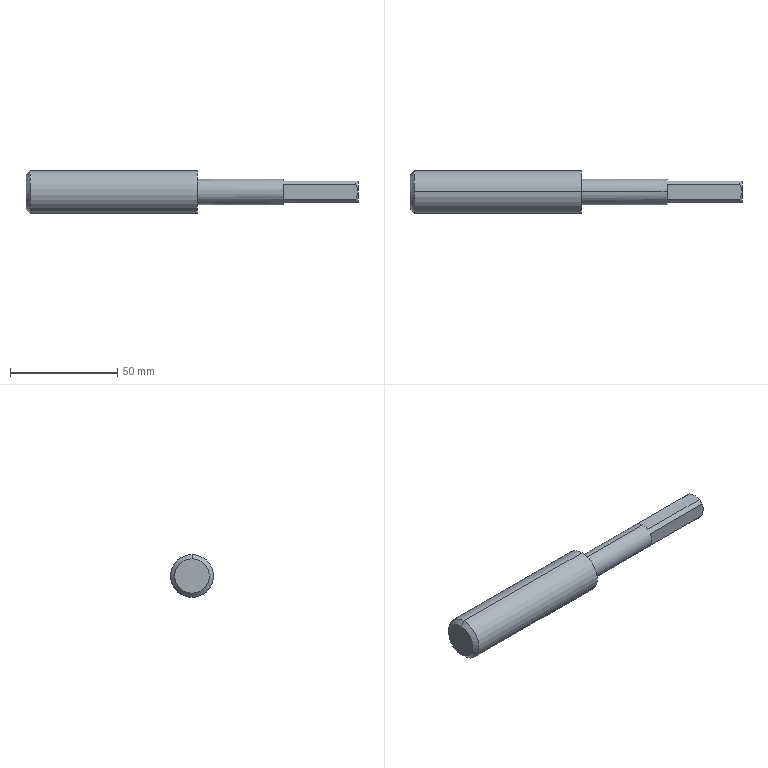Part | SolidWorks | features Chamfer 2, ICE 1, Revolution 1 | 1 solid | 21 faces | box 155 x 20 x 20 mm | volume 32861 mm3 | plane 11 | cone 6 | cylinder 4 | commonest cylinder face diameters 12 x2 20 x2
STEP:
#1=CARTESIAN_POINT('',(0.,0.,8.));
#2=VERTEX_POINT('',#1);
#3=CARTESIAN_POINT('',(0.,0.,-8.));
#4=VERTEX_POINT('',#3);
#5=CARTESIAN_POINT('',(0.,0.,0.));
#6=DIRECTION('',(-1.,0.,0.));
#7=DIRECTION('',(0.,0.,-1.));
#8=AXIS2_PLACEMENT_3D('',#5,#6,#7);
#9=CIRCLE('',#8,8.);
#10=EDGE_CURVE('',#2,#4,#9,.T.);
#11=ORIENTED_EDGE('',*,*,#10,.F.);
#12=CARTESIAN_POINT('',(2.,0.,10.));
#13=VERTEX_POINT('',#12);
#14=CARTESIAN_POINT('',(0.,0.,8.));
#15=DIRECTION('',(0.7071,0.,0.7071));
#16=VECTOR('',#15,1000.);
#17=LINE('',#14,#16);
#18=EDGE_CURVE('',#2,#13,#17,.T.);
#19=ORIENTED_EDGE('',*,*,#18,.T.);
#20=CARTESIAN_POINT('',(2.,0.,-10.));
#21=VERTEX_POINT('',#20);
#22=CARTESIAN_POINT('',(2.,0.,0.));
#23=DIRECTION('',(1.,0.,0.));
#24=DIRECTION('',(0.,0.,-1.));
#25=AXIS2_PLACEMENT_3D('',#22,#23,#24);
#26=CIRCLE('',#25,10.);
#27=EDGE_CURVE('',#21,#13,#26,.T.);
#28=ORIENTED_EDGE('',*,*,#27,.F.);
#29=CARTESIAN_POINT('',(0.,0.,-8.));
#30=DIRECTION('',(0.7071,0.,-0.7071));
#31=VECTOR('',#30,1000.);
#32=LINE('',#29,#31);
#33=EDGE_CURVE('',#4,#21,#32,.T.);
#34=ORIENTED_EDGE('',*,*,#33,.F.);
#35=EDGE_LOOP('',(#11,#19,#28,#34));
#36=FACE_OUTER_BOUND('',#35,.T.);
#37=CARTESIAN_POINT('',(0.,0.,0.));
#38=DIRECTION('',(1.,0.,0.));
#39=DIRECTION('',(0.,0.,-1.));
#40=AXIS2_PLACEMENT_3D('',#37,#38,#39);
#41=CONICAL_SURFACE('',#40,8.,0.7854);
#42=ADVANCED_FACE('',(#36),#41,.T.);
#43=CARTESIAN_POINT('',(80.,0.,10.));
#44=VERTEX_POINT('',#43);
#45=CARTESIAN_POINT('',(80.,0.,-10.));
#46=VERTEX_POINT('',#45);
#47=CARTESIAN_POINT('',(80.,0.,0.));
#48=DIRECTION('',(-1.,0.,0.));
#49=DIRECTION('',(0.,0.,1.));
#50=AXIS2_PLACEMENT_3D('',#47,#48,#49);
#51=CIRCLE('',#50,10.);
#52=EDGE_CURVE('',#44,#46,#51,.T.);
#53=ORIENTED_EDGE('',*,*,#52,.T.);
#54=CARTESIAN_POINT('',(0.,0.,-10.));
#55=DIRECTION('',(-1.,0.,0.));
#56=VECTOR('',#55,1000.);
#57=LINE('',#54,#56);
#58=EDGE_CURVE('',#46,#21,#57,.T.);
#59=ORIENTED_EDGE('',*,*,#58,.T.);
#60=ORIENTED_EDGE('',*,*,#27,.T.);
#61=CARTESIAN_POINT('',(0.,0.,10.));
#62=DIRECTION('',(-1.,0.,0.));
#63=VECTOR('',#62,1000.);
#64=LINE('',#61,#63);
#65=EDGE_CURVE('',#44,#13,#64,.T.);
#66=ORIENTED_EDGE('',*,*,#65,.F.);
#67=EDGE_LOOP('',(#53,#59,#60,#66));
#68=FACE_OUTER_BOUND('',#67,.T.);
#69=CARTESIAN_POINT('',(0.,0.,0.));
#70=DIRECTION('',(-1.,0.,0.));
#71=DIRECTION('',(0.,0.,1.));
#72=AXIS2_PLACEMENT_3D('',#69,#70,#71);
#73=CYLINDRICAL_SURFACE('',#72,10.);
#74=ADVANCED_FACE('',(#68),#73,.T.);
#75=CARTESIAN_POINT('',(120.,0.,-6.));
#76=VERTEX_POINT('',#75);
#77=CARTESIAN_POINT('',(120.,3.317,-5.));
#78=VERTEX_POINT('',#77);
#79=CARTESIAN_POINT('',(120.,0.,0.));
#80=DIRECTION('',(1.,0.,0.));
#81=DIRECTION('',(0.,0.,-1.));
#82=AXIS2_PLACEMENT_3D('',#79,#80,#81);
#83=CIRCLE('',#82,6.);
#84=EDGE_CURVE('',#76,#78,#83,.T.);
#85=ORIENTED_EDGE('',*,*,#84,.F.);
#86=CARTESIAN_POINT('',(80.,0.,-6.));
#87=VERTEX_POINT('',#86);
#88=CARTESIAN_POINT('',(0.,0.,-6.));
#89=DIRECTION('',(-1.,0.,0.));
#90=VECTOR('',#89,1000.);
#91=LINE('',#88,#90);
#92=EDGE_CURVE('',#76,#87,#91,.T.);
#93=ORIENTED_EDGE('',*,*,#92,.T.);
#94=CARTESIAN_POINT('',(80.,0.,6.));
#95=VERTEX_POINT('',#94);
#96=CARTESIAN_POINT('',(80.,0.,0.));
#97=DIRECTION('',(-1.,0.,0.));
#98=DIRECTION('',(0.,0.,1.));
#99=AXIS2_PLACEMENT_3D('',#96,#97,#98);
#100=CIRCLE('',#99,6.);
#101=EDGE_CURVE('',#95,#87,#100,.T.);
#102=ORIENTED_EDGE('',*,*,#101,.F.);
#103=CARTESIAN_POINT('',(120.,0.,6.));
#104=VERTEX_POINT('',#103);
#105=CARTESIAN_POINT('',(0.,0.,6.));
#106=DIRECTION('',(-1.,0.,0.));
#107=VECTOR('',#106,1000.);
#108=LINE('',#105,#107);
#109=EDGE_CURVE('',#104,#95,#108,.T.);
#110=ORIENTED_EDGE('',*,*,#109,.F.);
#111=CARTESIAN_POINT('',(120.,3.317,5.));
#112=VERTEX_POINT('',#111);
#113=CARTESIAN_POINT('',(120.,0.,0.));
#114=DIRECTION('',(1.,0.,0.));
#115=DIRECTION('',(0.,0.,-1.));
#116=AXIS2_PLACEMENT_3D('',#113,#114,#115);
#117=CIRCLE('',#116,6.);
#118=EDGE_CURVE('',#112,#104,#117,.T.);
#119=ORIENTED_EDGE('',*,*,#118,.F.);
#120=CARTESIAN_POINT('',(154.,3.317,5.));
#121=VERTEX_POINT('',#120);
#122=CARTESIAN_POINT('',(0.,3.317,5.));
#123=DIRECTION('',(-1.,0.,0.));
#124=VECTOR('',#123,1000.);
#125=LINE('',#122,#124);
#126=EDGE_CURVE('',#121,#112,#125,.T.);
#127=ORIENTED_EDGE('',*,*,#126,.F.);
#128=CARTESIAN_POINT('',(154.,5.,3.317));
#129=VERTEX_POINT('',#128);
#130=CARTESIAN_POINT('',(154.,0.,0.));
#131=DIRECTION('',(-1.,0.,0.));
#132=DIRECTION('',(0.,0.,1.));
#133=AXIS2_PLACEMENT_3D('',#130,#131,#132);
#134=CIRCLE('',#133,6.);
#135=EDGE_CURVE('',#121,#129,#134,.T.);
#136=ORIENTED_EDGE('',*,*,#135,.T.);
#137=CARTESIAN_POINT('',(120.,5.,3.317));
#138=VERTEX_POINT('',#137);
#139=CARTESIAN_POINT('',(0.,5.,3.317));
#140=DIRECTION('',(1.,0.,0.));
#141=VECTOR('',#140,1000.);
#142=LINE('',#139,#141);
#143=EDGE_CURVE('',#138,#129,#142,.T.);
#144=ORIENTED_EDGE('',*,*,#143,.F.);
#145=CARTESIAN_POINT('',(120.,5.,-3.317));
#146=VERTEX_POINT('',#145);
#147=CARTESIAN_POINT('',(120.,0.,0.));
#148=DIRECTION('',(1.,0.,0.));
#149=DIRECTION('',(0.,0.,-1.));
#150=AXIS2_PLACEMENT_3D('',#147,#148,#149);
#151=CIRCLE('',#150,6.);
#152=EDGE_CURVE('',#146,#138,#151,.T.);
#153=ORIENTED_EDGE('',*,*,#152,.F.);
#154=CARTESIAN_POINT('',(154.,5.,-3.317));
#155=VERTEX_POINT('',#154);
#156=CARTESIAN_POINT('',(0.,5.,-3.317));
#157=DIRECTION('',(-1.,0.,0.));
#158=VECTOR('',#157,1000.);
#159=LINE('',#156,#158);
#160=EDGE_CURVE('',#155,#146,#159,.T.);
#161=ORIENTED_EDGE('',*,*,#160,.F.);
#162=CARTESIAN_POINT('',(154.,3.317,-5.));
#163=VERTEX_POINT('',#162);
#164=CARTESIAN_POINT('',(154.,0.,0.));
#165=DIRECTION('',(-1.,0.,0.));
#166=DIRECTION('',(0.,0.,1.));
#167=AXIS2_PLACEMENT_3D('',#164,#165,#166);
#168=CIRCLE('',#167,6.);
#169=EDGE_CURVE('',#155,#163,#168,.T.);
#170=ORIENTED_EDGE('',*,*,#169,.T.);
#171=CARTESIAN_POINT('',(0.,3.317,-5.));
#172=DIRECTION('',(1.,0.,0.));
#173=VECTOR('',#172,1000.);
#174=LINE('',#171,#173);
#175=EDGE_CURVE('',#78,#163,#174,.T.);
#176=ORIENTED_EDGE('',*,*,#175,.F.);
#177=EDGE_LOOP('',(#85,#93,#102,#110,#119,#127,#136,#144,#153,#161,#170,#176));
#178=FACE_OUTER_BOUND('',#177,.T.);
#179=CARTESIAN_POINT('',(0.,0.,0.));
#180=DIRECTION('',(-1.,0.,0.));
#181=DIRECTION('',(0.,0.,1.));
#182=AXIS2_PLACEMENT_3D('',#179,#180,#181);
#183=CYLINDRICAL_SURFACE('',#182,6.);
#184=ADVANCED_FACE('',(#178),#183,.T.);
#185=ORIENTED_EDGE('',*,*,#92,.F.);
#186=CARTESIAN_POINT('',(120.,-3.317,-5.));
#187=VERTEX_POINT('',#186);
#188=CARTESIAN_POINT('',(120.,0.,0.));
#189=DIRECTION('',(1.,0.,0.));
#190=DIRECTION('',(0.,0.,-1.));
#191=AXIS2_PLACEMENT_3D('',#188,#189,#190);
#192=CIRCLE('',#191,6.);
#193=EDGE_CURVE('',#187,#76,#192,.T.);
#194=ORIENTED_EDGE('',*,*,#193,.F.);
#195=CARTESIAN_POINT('',(154.,-3.317,-5.));
#196=VERTEX_POINT('',#195);
#197=CARTESIAN_POINT('',(0.,-3.317,-5.));
#198=DIRECTION('',(-1.,0.,0.));
#199=VECTOR('',#198,1000.);
#200=LINE('',#197,#199);
#201=EDGE_CURVE('',#196,#187,#200,.T.);
#202=ORIENTED_EDGE('',*,*,#201,.F.);
#203=CARTESIAN_POINT('',(154.,-5.,-3.317));
#204=VERTEX_POINT('',#203);
#205=CARTESIAN_POINT('',(154.,0.,0.));
#206=DIRECTION('',(-1.,0.,0.));
#207=DIRECTION('',(0.,0.,1.));
#208=AXIS2_PLACEMENT_3D('',#205,#206,#207);
#209=CIRCLE('',#208,6.);
#210=EDGE_CURVE('',#196,#204,#209,.T.);
#211=ORIENTED_EDGE('',*,*,#210,.T.);
#212=CARTESIAN_POINT('',(120.,-5.,-3.317));
#213=VERTEX_POINT('',#212);
#214=CARTESIAN_POINT('',(0.,-5.,-3.317));
#215=DIRECTION('',(1.,0.,0.));
#216=VECTOR('',#215,1000.);
#217=LINE('',#214,#216);
#218=EDGE_CURVE('',#213,#204,#217,.T.);
#219=ORIENTED_EDGE('',*,*,#218,.F.);
#220=CARTESIAN_POINT('',(120.,-5.,3.317));
#221=VERTEX_POINT('',#220);
#222=CARTESIAN_POINT('',(120.,0.,0.));
#223=DIRECTION('',(1.,0.,0.));
#224=DIRECTION('',(0.,0.,-1.));
#225=AXIS2_PLACEMENT_3D('',#222,#223,#224);
#226=CIRCLE('',#225,6.);
#227=EDGE_CURVE('',#221,#213,#226,.T.);
#228=ORIENTED_EDGE('',*,*,#227,.F.);
#229=CARTESIAN_POINT('',(154.,-5.,3.317));
#230=VERTEX_POINT('',#229);
#231=CARTESIAN_POINT('',(0.,-5.,3.317));
#232=DIRECTION('',(-1.,0.,0.));
#233=VECTOR('',#232,1000.);
#234=LINE('',#231,#233);
#235=EDGE_CURVE('',#230,#221,#234,.T.);
#236=ORIENTED_EDGE('',*,*,#235,.F.);
#237=CARTESIAN_POINT('',(154.,-3.317,5.));
#238=VERTEX_POINT('',#237);
#239=CARTESIAN_POINT('',(154.,0.,0.));
#240=DIRECTION('',(-1.,0.,0.));
#241=DIRECTION('',(0.,0.,1.));
#242=AXIS2_PLACEMENT_3D('',#239,#240,#241);
#243=CIRCLE('',#242,6.);
#244=EDGE_CURVE('',#230,#238,#243,.T.);
#245=ORIENTED_EDGE('',*,*,#244,.T.);
#246=CARTESIAN_POINT('',(120.,-3.317,5.));
#247=VERTEX_POINT('',#246);
#248=CARTESIAN_POINT('',(0.,-3.317,5.));
#249=DIRECTION('',(1.,0.,0.));
#250=VECTOR('',#249,1000.);
#251=LINE('',#248,#250);
#252=EDGE_CURVE('',#247,#238,#251,.T.);
#253=ORIENTED_EDGE('',*,*,#252,.F.);
#254=CARTESIAN_POINT('',(120.,0.,0.));
#255=DIRECTION('',(1.,0.,0.));
#256=DIRECTION('',(0.,0.,-1.));
#257=AXIS2_PLACEMENT_3D('',#254,#255,#256);
#258=CIRCLE('',#257,6.);
#259=EDGE_CURVE('',#104,#247,#258,.T.);
#260=ORIENTED_EDGE('',*,*,#259,.F.);
#261=ORIENTED_EDGE('',*,*,#109,.T.);
#262=CARTESIAN_POINT('',(80.,0.,0.));
#263=DIRECTION('',(-1.,0.,0.));
#264=DIRECTION('',(0.,0.,1.));
#265=AXIS2_PLACEMENT_3D('',#262,#263,#264);
#266=CIRCLE('',#265,6.);
#267=EDGE_CURVE('',#87,#95,#266,.T.);
#268=ORIENTED_EDGE('',*,*,#267,.F.);
#269=EDGE_LOOP('',(#185,#194,#202,#211,#219,#228,#236,#245,#253,#260,#261,#268));
#270=FACE_OUTER_BOUND('',#269,.T.);
#271=CARTESIAN_POINT('',(0.,0.,0.));
#272=DIRECTION('',(-1.,0.,0.));
#273=DIRECTION('',(0.,0.,1.));
#274=AXIS2_PLACEMENT_3D('',#271,#272,#273);
#275=CYLINDRICAL_SURFACE('',#274,6.);
#276=ADVANCED_FACE('',(#270),#275,.T.);
#277=ORIENTED_EDGE('',*,*,#210,.F.);
#278=CARTESIAN_POINT('',(155.,0.,-5.));
#279=VERTEX_POINT('',#278);
#280=CARTESIAN_POINT('',(154.,-3.317,-5.));
#281=CARTESIAN_POINT('',(154.283,-2.804,-5.));
#282=CARTESIAN_POINT('',(154.531,-2.277,-5.));
#283=CARTESIAN_POINT('',(154.802,-1.445,-5.));
#284=CARTESIAN_POINT('',(154.875,-1.159,-5.));
#285=CARTESIAN_POINT('',(154.974,-0.581,-5.));
#286=CARTESIAN_POINT('',(155.,-0.2911,-5.));
#287=CARTESIAN_POINT('',(155.,0.,-5.));
#288=B_SPLINE_CURVE_WITH_KNOTS('',3,(#280,#281,#282,#283,#284,#285,#286,#287),.UNSPECIFIED.,.F.,.F.,(4,2,2,4),(0.007275,0.009018,0.009889,0.01076),.UNSPECIFIED.);
#289=EDGE_CURVE('',#196,#279,#288,.T.);
#290=ORIENTED_EDGE('',*,*,#289,.T.);
#291=CARTESIAN_POINT('',(155.,-5.,0.));
#292=VERTEX_POINT('',#291);
#293=CARTESIAN_POINT('',(155.,0.,0.));
#294=DIRECTION('',(1.,0.,0.));
#295=DIRECTION('',(0.,0.,1.));
#296=AXIS2_PLACEMENT_3D('',#293,#294,#295);
#297=CIRCLE('',#296,5.);
#298=EDGE_CURVE('',#292,#279,#297,.T.);
#299=ORIENTED_EDGE('',*,*,#298,.F.);
#300=CARTESIAN_POINT('',(155.,-5.,0.));
#301=CARTESIAN_POINT('',(155.,-5.,-0.2911));
#302=CARTESIAN_POINT('',(154.974,-5.,-0.581));
#303=CARTESIAN_POINT('',(154.875,-5.,-1.159));
#304=CARTESIAN_POINT('',(154.802,-5.,-1.445));
#305=CARTESIAN_POINT('',(154.531,-5.,-2.277));
#306=CARTESIAN_POINT('',(154.283,-5.,-2.804));
#307=CARTESIAN_POINT('',(154.,-5.,-3.317));
#308=B_SPLINE_CURVE_WITH_KNOTS('',3,(#300,#301,#302,#303,#304,#305,#306,#307),.UNSPECIFIED.,.F.,.F.,(4,2,2,4),(0.01182,0.01268,0.01355,0.01528),.UNSPECIFIED.);
#309=EDGE_CURVE('',#292,#204,#308,.T.);
#310=ORIENTED_EDGE('',*,*,#309,.T.);
#311=EDGE_LOOP('',(#277,#290,#299,#310));
#312=FACE_OUTER_BOUND('',#311,.T.);
#313=CARTESIAN_POINT('',(154.,0.,0.));
#314=DIRECTION('',(-1.,0.,0.));
#315=DIRECTION('',(0.,0.,1.));
#316=AXIS2_PLACEMENT_3D('',#313,#314,#315);
#317=CONICAL_SURFACE('',#316,6.,0.7854);
#318=ADVANCED_FACE('',(#312),#317,.T.);
#319=CARTESIAN_POINT('',(155.,5.,0.));
#320=VERTEX_POINT('',#319);
#321=CARTESIAN_POINT('',(155.,0.,0.));
#322=DIRECTION('',(1.,0.,0.));
#323=DIRECTION('',(0.,0.,1.));
#324=AXIS2_PLACEMENT_3D('',#321,#322,#323);
#325=CIRCLE('',#324,5.);
#326=EDGE_CURVE('',#279,#320,#325,.T.);
#327=ORIENTED_EDGE('',*,*,#326,.F.);
#328=CARTESIAN_POINT('',(155.,0.,-5.));
#329=CARTESIAN_POINT('',(155.,0.2907,-5.));
#330=CARTESIAN_POINT('',(154.974,0.5851,-5.));
#331=CARTESIAN_POINT('',(154.874,1.163,-5.));
#332=CARTESIAN_POINT('',(154.802,1.445,-5.));
#333=CARTESIAN_POINT('',(154.622,1.997,-5.));
#334=CARTESIAN_POINT('',(154.515,2.268,-5.));
#335=CARTESIAN_POINT('',(154.274,2.801,-5.));
#336=CARTESIAN_POINT('',(154.141,3.062,-5.));
#337=CARTESIAN_POINT('',(154.,3.317,-5.));
#338=B_SPLINE_CURVE_WITH_KNOTS('',3,(#328,#329,#330,#331,#332,#333,#334,#335,#336,#337),.UNSPECIFIED.,.F.,.F.,(4,2,2,2,4),(0.01076,0.01163,0.0125,0.01337,0.01424),.UNSPECIFIED.);
#339=EDGE_CURVE('',#279,#163,#338,.T.);
#340=ORIENTED_EDGE('',*,*,#339,.T.);
#341=ORIENTED_EDGE('',*,*,#169,.F.);
#342=CARTESIAN_POINT('',(154.,5.,-3.317));
#343=CARTESIAN_POINT('',(154.283,5.,-2.804));
#344=CARTESIAN_POINT('',(154.531,5.,-2.277));
#345=CARTESIAN_POINT('',(154.802,5.,-1.445));
#346=CARTESIAN_POINT('',(154.875,5.,-1.159));
#347=CARTESIAN_POINT('',(154.974,5.,-0.581));
#348=CARTESIAN_POINT('',(155.,5.,-0.2911));
#349=CARTESIAN_POINT('',(155.,5.,0.));
#350=B_SPLINE_CURVE_WITH_KNOTS('',3,(#342,#343,#344,#345,#346,#347,#348,#349),.UNSPECIFIED.,.F.,.F.,(4,2,2,4),(0.007275,0.009018,0.009889,0.01076),.UNSPECIFIED.);
#351=EDGE_CURVE('',#155,#320,#350,.T.);
#352=ORIENTED_EDGE('',*,*,#351,.T.);
#353=EDGE_LOOP('',(#327,#340,#341,#352));
#354=FACE_OUTER_BOUND('',#353,.T.);
#355=CARTESIAN_POINT('',(154.,0.,0.));
#356=DIRECTION('',(-1.,0.,0.));
#357=DIRECTION('',(0.,0.,1.));
#358=AXIS2_PLACEMENT_3D('',#355,#356,#357);
#359=CONICAL_SURFACE('',#358,6.,0.7854);
#360=ADVANCED_FACE('',(#354),#359,.T.);
#361=ORIENTED_EDGE('',*,*,#244,.F.);
#362=CARTESIAN_POINT('',(154.,-5.,3.317));
#363=CARTESIAN_POINT('',(154.141,-5.,3.062));
#364=CARTESIAN_POINT('',(154.274,-5.,2.801));
#365=CARTESIAN_POINT('',(154.515,-5.,2.268));
#366=CARTESIAN_POINT('',(154.622,-5.,1.997));
#367=CARTESIAN_POINT('',(154.802,-5.,1.445));
#368=CARTESIAN_POINT('',(154.874,-5.,1.163));
#369=CARTESIAN_POINT('',(154.974,-5.,0.5851));
#370=CARTESIAN_POINT('',(155.,-5.,0.2907));
#371=CARTESIAN_POINT('',(155.,-5.,0.));
#372=B_SPLINE_CURVE_WITH_KNOTS('',3,(#362,#363,#364,#365,#366,#367,#368,#369,#370,#371),.UNSPECIFIED.,.F.,.F.,(4,2,2,2,4),(0.008366,0.009229,0.01009,0.01096,0.01182),.UNSPECIFIED.);
#373=EDGE_CURVE('',#230,#292,#372,.T.);
#374=ORIENTED_EDGE('',*,*,#373,.T.);
#375=CARTESIAN_POINT('',(155.,0.,5.));
#376=VERTEX_POINT('',#375);
#377=CARTESIAN_POINT('',(155.,0.,0.));
#378=DIRECTION('',(1.,0.,0.));
#379=DIRECTION('',(0.,0.,1.));
#380=AXIS2_PLACEMENT_3D('',#377,#378,#379);
#381=CIRCLE('',#380,5.);
#382=EDGE_CURVE('',#376,#292,#381,.T.);
#383=ORIENTED_EDGE('',*,*,#382,.F.);
#384=CARTESIAN_POINT('',(155.,0.,5.));
#385=CARTESIAN_POINT('',(155.,-0.2911,5.));
#386=CARTESIAN_POINT('',(154.974,-0.581,5.));
#387=CARTESIAN_POINT('',(154.875,-1.159,5.));
#388=CARTESIAN_POINT('',(154.802,-1.445,5.));
#389=CARTESIAN_POINT('',(154.531,-2.277,5.));
#390=CARTESIAN_POINT('',(154.283,-2.804,5.));
#391=CARTESIAN_POINT('',(154.,-3.317,5.));
#392=B_SPLINE_CURVE_WITH_KNOTS('',3,(#384,#385,#386,#387,#388,#389,#390,#391),.UNSPECIFIED.,.F.,.F.,(4,2,2,4),(0.01182,0.01268,0.01355,0.01528),.UNSPECIFIED.);
#393=EDGE_CURVE('',#376,#238,#392,.T.);
#394=ORIENTED_EDGE('',*,*,#393,.T.);
#395=EDGE_LOOP('',(#361,#374,#383,#394));
#396=FACE_OUTER_BOUND('',#395,.T.);
#397=CARTESIAN_POINT('',(154.,0.,0.));
#398=DIRECTION('',(-1.,0.,0.));
#399=DIRECTION('',(0.,0.,1.));
#400=AXIS2_PLACEMENT_3D('',#397,#398,#399);
#401=CONICAL_SURFACE('',#400,6.,0.7854);
#402=ADVANCED_FACE('',(#396),#401,.T.);
#403=ORIENTED_EDGE('',*,*,#135,.F.);
#404=CARTESIAN_POINT('',(154.,3.317,5.));
#405=CARTESIAN_POINT('',(154.141,3.062,5.));
#406=CARTESIAN_POINT('',(154.274,2.801,5.));
#407=CARTESIAN_POINT('',(154.515,2.268,5.));
#408=CARTESIAN_POINT('',(154.622,1.997,5.));
#409=CARTESIAN_POINT('',(154.802,1.445,5.));
#410=CARTESIAN_POINT('',(154.874,1.163,5.));
#411=CARTESIAN_POINT('',(154.974,0.5851,5.));
#412=CARTESIAN_POINT('',(155.,0.2907,5.));
#413=CARTESIAN_POINT('',(155.,0.,5.));
#414=B_SPLINE_CURVE_WITH_KNOTS('',3,(#404,#405,#406,#407,#408,#409,#410,#411,#412,#413),.UNSPECIFIED.,.F.,.F.,(4,2,2,2,4),(0.008366,0.009229,0.01009,0.01096,0.01182),.UNSPECIFIED.);
#415=EDGE_CURVE('',#121,#376,#414,.T.);
#416=ORIENTED_EDGE('',*,*,#415,.T.);
#417=CARTESIAN_POINT('',(155.,0.,0.));
#418=DIRECTION('',(1.,0.,0.));
#419=DIRECTION('',(0.,0.,1.));
#420=AXIS2_PLACEMENT_3D('',#417,#418,#419);
#421=CIRCLE('',#420,5.);
#422=EDGE_CURVE('',#320,#376,#421,.T.);
#423=ORIENTED_EDGE('',*,*,#422,.F.);
#424=CARTESIAN_POINT('',(155.,5.,0.));
#425=CARTESIAN_POINT('',(155.,5.,0.2907));
#426=CARTESIAN_POINT('',(154.974,5.,0.5851));
#427=CARTESIAN_POINT('',(154.874,5.,1.163));
#428=CARTESIAN_POINT('',(154.802,5.,1.445));
#429=CARTESIAN_POINT('',(154.622,5.,1.997));
#430=CARTESIAN_POINT('',(154.515,5.,2.268));
#431=CARTESIAN_POINT('',(154.274,5.,2.801));
#432=CARTESIAN_POINT('',(154.141,5.,3.062));
#433=CARTESIAN_POINT('',(154.,5.,3.317));
#434=B_SPLINE_CURVE_WITH_KNOTS('',3,(#424,#425,#426,#427,#428,#429,#430,#431,#432,#433),.UNSPECIFIED.,.F.,.F.,(4,2,2,2,4),(0.01076,0.01163,0.0125,0.01337,0.01424),.UNSPECIFIED.);
#435=EDGE_CURVE('',#320,#129,#434,.T.);
#436=ORIENTED_EDGE('',*,*,#435,.T.);
#437=EDGE_LOOP('',(#403,#416,#423,#436));
#438=FACE_OUTER_BOUND('',#437,.T.);
#439=CARTESIAN_POINT('',(154.,0.,0.));
#440=DIRECTION('',(-1.,0.,0.));
#441=DIRECTION('',(0.,0.,1.));
#442=AXIS2_PLACEMENT_3D('',#439,#440,#441);
#443=CONICAL_SURFACE('',#442,6.,0.7854);
#444=ADVANCED_FACE('',(#438),#443,.T.);
#445=CARTESIAN_POINT('',(0.,0.,0.));
#446=DIRECTION('',(-1.,0.,0.));
#447=DIRECTION('',(0.,0.,-1.));
#448=AXIS2_PLACEMENT_3D('',#445,#446,#447);
#449=CIRCLE('',#448,8.);
#450=EDGE_CURVE('',#4,#2,#449,.T.);
#451=ORIENTED_EDGE('',*,*,#450,.T.);
#452=ORIENTED_EDGE('',*,*,#10,.T.);
#453=EDGE_LOOP('',(#451,#452));
#454=FACE_OUTER_BOUND('',#453,.T.);
#455=CARTESIAN_POINT('',(0.,0.,0.));
#456=DIRECTION('',(1.,0.,0.));
#457=DIRECTION('',(0.,0.,-1.));
#458=AXIS2_PLACEMENT_3D('',#455,#456,#457);
#459=PLANE('',#458);
#460=ADVANCED_FACE('',(#454),#459,.F.);
#461=ORIENTED_EDGE('',*,*,#58,.F.);
#462=CARTESIAN_POINT('',(80.,0.,0.));
#463=DIRECTION('',(-1.,0.,0.));
#464=DIRECTION('',(0.,0.,1.));
#465=AXIS2_PLACEMENT_3D('',#462,#463,#464);
#466=CIRCLE('',#465,10.);
#467=EDGE_CURVE('',#46,#44,#466,.T.);
#468=ORIENTED_EDGE('',*,*,#467,.T.);
#469=ORIENTED_EDGE('',*,*,#65,.T.);
#470=CARTESIAN_POINT('',(2.,0.,0.));
#471=DIRECTION('',(1.,0.,0.));
#472=DIRECTION('',(0.,0.,-1.));
#473=AXIS2_PLACEMENT_3D('',#470,#471,#472);
#474=CIRCLE('',#473,10.);
#475=EDGE_CURVE('',#13,#21,#474,.T.);
#476=ORIENTED_EDGE('',*,*,#475,.T.);
#477=EDGE_LOOP('',(#461,#468,#469,#476));
#478=FACE_OUTER_BOUND('',#477,.T.);
#479=CARTESIAN_POINT('',(0.,0.,0.));
#480=DIRECTION('',(-1.,0.,0.));
#481=DIRECTION('',(0.,0.,1.));
#482=AXIS2_PLACEMENT_3D('',#479,#480,#481);
#483=CYLINDRICAL_SURFACE('',#482,10.);
#484=ADVANCED_FACE('',(#478),#483,.T.);
#485=ORIENTED_EDGE('',*,*,#52,.F.);
#486=ORIENTED_EDGE('',*,*,#467,.F.);
#487=EDGE_LOOP('',(#485,#486));
#488=FACE_OUTER_BOUND('',#487,.T.);
#489=ORIENTED_EDGE('',*,*,#101,.T.);
#490=ORIENTED_EDGE('',*,*,#267,.T.);
#491=EDGE_LOOP('',(#489,#490));
#492=FACE_BOUND('',#491,.T.);
#493=CARTESIAN_POINT('',(80.,10.,0.));
#494=DIRECTION('',(-1.,0.,0.));
#495=DIRECTION('',(0.,0.,1.));
#496=AXIS2_PLACEMENT_3D('',#493,#494,#495);
#497=PLANE('',#496);
#498=ADVANCED_FACE('',(#488,#492),#497,.F.);
#499=ORIENTED_EDGE('',*,*,#382,.T.);
#500=ORIENTED_EDGE('',*,*,#298,.T.);
#501=ORIENTED_EDGE('',*,*,#326,.T.);
#502=ORIENTED_EDGE('',*,*,#422,.T.);
#503=EDGE_LOOP('',(#499,#500,#501,#502));
#504=FACE_OUTER_BOUND('',#503,.T.);
#505=CARTESIAN_POINT('',(155.,6.,0.));
#506=DIRECTION('',(-1.,0.,0.));
#507=DIRECTION('',(0.,0.,1.));
#508=AXIS2_PLACEMENT_3D('',#505,#506,#507);
#509=PLANE('',#508);
#510=ADVANCED_FACE('',(#504),#509,.F.);
#511=ORIENTED_EDGE('',*,*,#18,.F.);
#512=ORIENTED_EDGE('',*,*,#450,.F.);
#513=ORIENTED_EDGE('',*,*,#33,.T.);
#514=ORIENTED_EDGE('',*,*,#475,.F.);
#515=EDGE_LOOP('',(#511,#512,#513,#514));
#516=FACE_OUTER_BOUND('',#515,.T.);
#517=CARTESIAN_POINT('',(0.,0.,0.));
#518=DIRECTION('',(1.,0.,0.));
#519=DIRECTION('',(0.,0.,-1.));
#520=AXIS2_PLACEMENT_3D('',#517,#518,#519);
#521=CONICAL_SURFACE('',#520,8.,0.7854);
#522=ADVANCED_FACE('',(#516),#521,.T.);
#523=ORIENTED_EDGE('',*,*,#160,.T.);
#524=CARTESIAN_POINT('',(120.,5.,5.));
#525=DIRECTION('',(0.,0.,1.));
#526=VECTOR('',#525,1000.);
#527=LINE('',#524,#526);
#528=EDGE_CURVE('',#146,#138,#527,.T.);
#529=ORIENTED_EDGE('',*,*,#528,.T.);
#530=ORIENTED_EDGE('',*,*,#143,.T.);
#531=ORIENTED_EDGE('',*,*,#435,.F.);
#532=ORIENTED_EDGE('',*,*,#351,.F.);
#533=EDGE_LOOP('',(#523,#529,#530,#531,#532));
#534=FACE_OUTER_BOUND('',#533,.T.);
#535=CARTESIAN_POINT('',(120.,5.,5.));
#536=DIRECTION('',(0.,1.,0.));
#537=DIRECTION('',(0.,0.,1.));
#538=AXIS2_PLACEMENT_3D('',#535,#536,#537);
#539=PLANE('',#538);
#540=ADVANCED_FACE('',(#534),#539,.T.);
#541=ORIENTED_EDGE('',*,*,#152,.T.);
#542=ORIENTED_EDGE('',*,*,#528,.F.);
#543=EDGE_LOOP('',(#541,#542));
#544=FACE_OUTER_BOUND('',#543,.T.);
#545=CARTESIAN_POINT('',(120.,0.,0.));
#546=DIRECTION('',(1.,0.,0.));
#547=DIRECTION('',(0.,0.,-1.));
#548=AXIS2_PLACEMENT_3D('',#545,#546,#547);
#549=PLANE('',#548);
#550=ADVANCED_FACE('',(#544),#549,.T.);
#551=ORIENTED_EDGE('',*,*,#126,.T.);
#552=CARTESIAN_POINT('',(120.,-5.,5.));
#553=DIRECTION('',(0.,-1.,0.));
#554=VECTOR('',#553,1000.);
#555=LINE('',#552,#554);
#556=EDGE_CURVE('',#112,#247,#555,.T.);
#557=ORIENTED_EDGE('',*,*,#556,.T.);
#558=ORIENTED_EDGE('',*,*,#252,.T.);
#559=ORIENTED_EDGE('',*,*,#393,.F.);
#560=ORIENTED_EDGE('',*,*,#415,.F.);
#561=EDGE_LOOP('',(#551,#557,#558,#559,#560));
#562=FACE_OUTER_BOUND('',#561,.T.);
#563=CARTESIAN_POINT('',(120.,-5.,5.));
#564=DIRECTION('',(0.,0.,1.));
#565=DIRECTION('',(1.,0.,0.));
#566=AXIS2_PLACEMENT_3D('',#563,#564,#565);
#567=PLANE('',#566);
#568=ADVANCED_FACE('',(#562),#567,.T.);
#569=ORIENTED_EDGE('',*,*,#118,.T.);
#570=ORIENTED_EDGE('',*,*,#259,.T.);
#571=ORIENTED_EDGE('',*,*,#556,.F.);
#572=EDGE_LOOP('',(#569,#570,#571));
#573=FACE_OUTER_BOUND('',#572,.T.);
#574=CARTESIAN_POINT('',(120.,0.,0.));
#575=DIRECTION('',(1.,0.,0.));
#576=DIRECTION('',(0.,0.,-1.));
#577=AXIS2_PLACEMENT_3D('',#574,#575,#576);
#578=PLANE('',#577);
#579=ADVANCED_FACE('',(#573),#578,.T.);
#580=ORIENTED_EDGE('',*,*,#235,.T.);
#581=CARTESIAN_POINT('',(120.,-5.,5.));
#582=DIRECTION('',(0.,0.,-1.));
#583=VECTOR('',#582,1000.);
#584=LINE('',#581,#583);
#585=EDGE_CURVE('',#221,#213,#584,.T.);
#586=ORIENTED_EDGE('',*,*,#585,.T.);
#587=ORIENTED_EDGE('',*,*,#218,.T.);
#588=ORIENTED_EDGE('',*,*,#309,.F.);
#589=ORIENTED_EDGE('',*,*,#373,.F.);
#590=EDGE_LOOP('',(#580,#586,#587,#588,#589));
#591=FACE_OUTER_BOUND('',#590,.T.);
#592=CARTESIAN_POINT('',(120.,-5.,5.));
#593=DIRECTION('',(0.,-1.,0.));
#594=DIRECTION('',(0.,0.,-1.));
#595=AXIS2_PLACEMENT_3D('',#592,#593,#594);
#596=PLANE('',#595);
#597=ADVANCED_FACE('',(#591),#596,.T.);
#598=ORIENTED_EDGE('',*,*,#227,.T.);
#599=ORIENTED_EDGE('',*,*,#585,.F.);
#600=EDGE_LOOP('',(#598,#599));
#601=FACE_OUTER_BOUND('',#600,.T.);
#602=CARTESIAN_POINT('',(120.,0.,0.));
#603=DIRECTION('',(1.,0.,0.));
#604=DIRECTION('',(0.,0.,-1.));
#605=AXIS2_PLACEMENT_3D('',#602,#603,#604);
#606=PLANE('',#605);
#607=ADVANCED_FACE('',(#601),#606,.T.);
#608=ORIENTED_EDGE('',*,*,#193,.T.);
#609=ORIENTED_EDGE('',*,*,#84,.T.);
#610=CARTESIAN_POINT('',(120.,-5.,-5.));
#611=DIRECTION('',(0.,1.,0.));
#612=VECTOR('',#611,1000.);
#613=LINE('',#610,#612);
#614=EDGE_CURVE('',#187,#78,#613,.T.);
#615=ORIENTED_EDGE('',*,*,#614,.F.);
#616=EDGE_LOOP('',(#608,#609,#615));
#617=FACE_OUTER_BOUND('',#616,.T.);
#618=CARTESIAN_POINT('',(120.,0.,0.));
#619=DIRECTION('',(1.,0.,0.));
#620=DIRECTION('',(0.,0.,-1.));
#621=AXIS2_PLACEMENT_3D('',#618,#619,#620);
#622=PLANE('',#621);
#623=ADVANCED_FACE('',(#617),#622,.T.);
#624=ORIENTED_EDGE('',*,*,#201,.T.);
#625=ORIENTED_EDGE('',*,*,#614,.T.);
#626=ORIENTED_EDGE('',*,*,#175,.T.);
#627=ORIENTED_EDGE('',*,*,#339,.F.);
#628=ORIENTED_EDGE('',*,*,#289,.F.);
#629=EDGE_LOOP('',(#624,#625,#626,#627,#628));
#630=FACE_OUTER_BOUND('',#629,.T.);
#631=CARTESIAN_POINT('',(120.,-5.,-5.));
#632=DIRECTION('',(0.,0.,-1.));
#633=DIRECTION('',(-1.,0.,0.));
#634=AXIS2_PLACEMENT_3D('',#631,#632,#633);
#635=PLANE('',#634);
#636=ADVANCED_FACE('',(#630),#635,.T.);
#637=CLOSED_SHELL('',(#42,#74,#184,#276,#318,#360,#402,#444,#460,#484,#498,#510,#522,#540,#550,#568,#579,#597,#607,#623,#636));
#638=MANIFOLD_SOLID_BREP('',#637);
#639=CARTESIAN_POINT('',(0.,0.,0.));
#640=DIRECTION('',(0.,0.,1.));
#641=DIRECTION('',(1.,0.,0.));
#642=AXIS2_PLACEMENT_3D('',#639,#640,#641);
#643=(LENGTH_UNIT()NAMED_UNIT(*)SI_UNIT(.MILLI.,.METRE.));
#644=UNCERTAINTY_MEASURE_WITH_UNIT(LENGTH_MEASURE(0.00001),#643,'','');
#645=(NAMED_UNIT(*)PLANE_ANGLE_UNIT()SI_UNIT($,.RADIAN.));
#646=(NAMED_UNIT(*)SI_UNIT($,.STERADIAN.)SOLID_ANGLE_UNIT());
#647=(GEOMETRIC_REPRESENTATION_CONTEXT(3)GLOBAL_UNCERTAINTY_ASSIGNED_CONTEXT((#644))GLOBAL_UNIT_ASSIGNED_CONTEXT((#643,#645,#646))REPRESENTATION_CONTEXT('',''));
#648=ADVANCED_BREP_SHAPE_REPRESENTATION('',(#638,#642),#647);